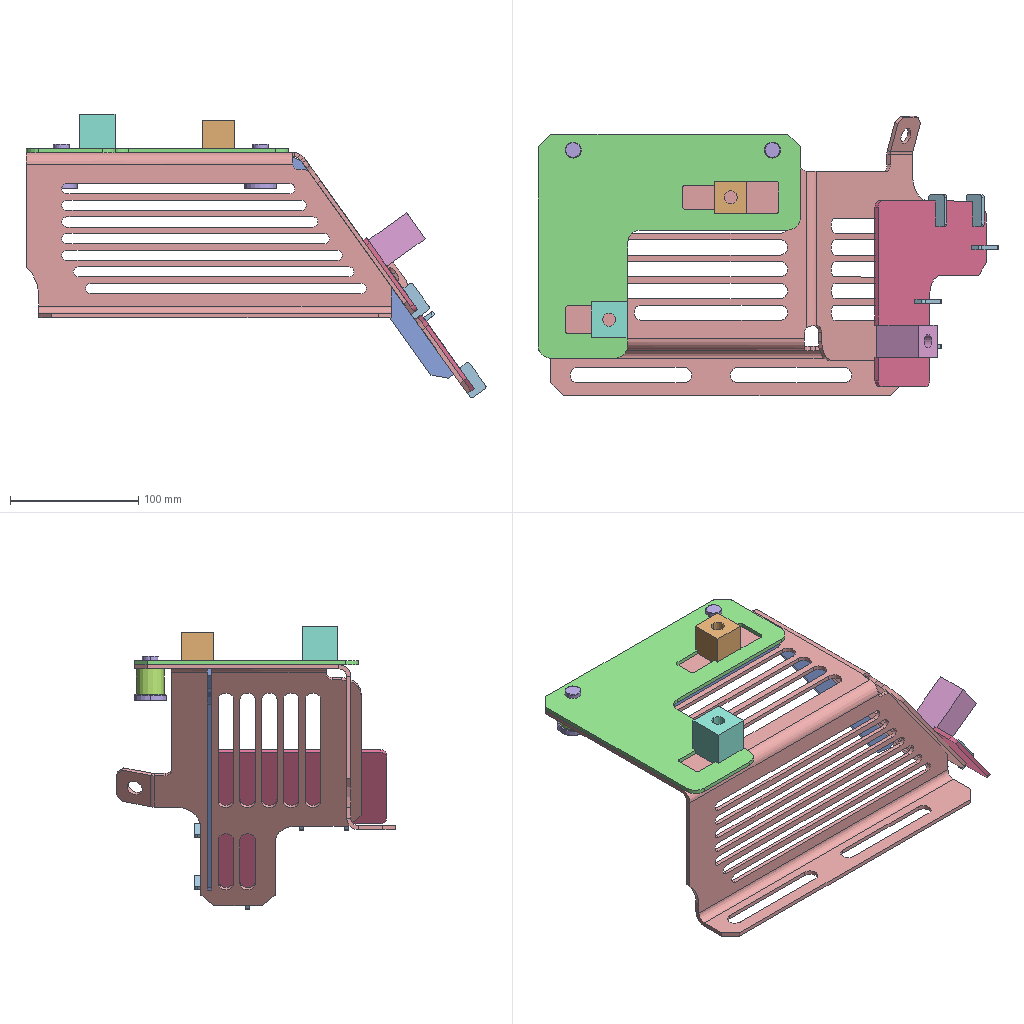Assembly | SolidWorks | 10 different items | 16 placed | box 359 x 218 x 221 mm
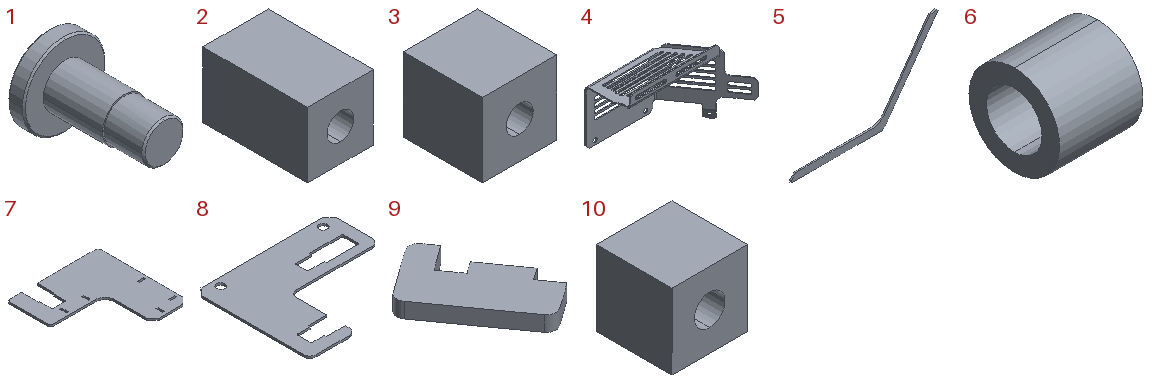Parts list (item | quantity | size | volume | features):
1 | x2 | 25 x 35 x 25 mm | 6404 mm3 | features Chamfer 1, Revolution 1
2 | x1 | 25 x 40 x 25 mm | 21731 mm3 | features FlatPattern 1, HoleWzd 1, SMBaseFlange 1, SheetMetal 1
3 | x1 | 28 x 30 x 28 mm | 21069 mm3 | features Extrusion 1, HoleWzd 1
4 | x1 | 347.398 x 187.972 x 217.987 mm | 228899 mm3 | features SM3dBend 4, FlatPattern 1, SMBaseFlange 1, SheetMetal 1
5 | x1 | 326.5 x 3.2 x 172.806 mm | 19256 mm3 | features FlatPattern 1, SMBaseFlange 1, SheetMetal 1
6 | x2 | 20 x 21.7 x 21.7 mm | 4618 mm3 | features Extrusion 1
7 | x1 | 145 x 145 x 3.2 mm | 41790 mm3 | features FlatPattern 1, SMBaseFlange 1, SheetMetal 1
8 | x1 | 205 x 175 x 3.2 mm | 60892 mm3 | features FlatPattern 1, SMBaseFlange 1, SheetMetal 1
9 | x5 | 20.748 x 27.48 x 3.2 mm | 878.159 mm3 | features FlatPattern 1, SMBaseFlange 1, SheetMetal 1
10 | x1 | 25 x 25 x 25 mm | 13582 mm3 | features Extrusion 1, HoleWzd 1
Mates (type | each side: item.copy, entity, surface, feature):
Coincident | 4.1 face plane Base-Flange1 | 5.1 face plane Base-Flange1 | 2 times
DistanceDim | 4.1 face plane Base-Flange1 | 5.1 face plane Base-Flange1
Coincident | 4.1 face plane Base-Flange1 | 6.1 face plane Boss-Extrude1
Concentric | 4.1 face cylinder Base-Flange1 | 6.1 face cylinder Boss-Extrude1
Coincident | 4.1 face plane Base-Flange1 | 6.2 face plane Boss-Extrude1
Concentric | 4.1 face cylinder Base-Flange1 | 6.2 face cylinder Boss-Extrude1
Coincident | 4.1 face plane Base-Flange1 | 2.1 face plane Base-Flange1
DistanceDim | 2.1 face plane Base-Flange1 | 4.1 face plane Base-Flange1
DistanceDim | 4.1 face plane Base-Flange1 | 2.1 face plane Base-Flange1
Coincident | 4.1 face plane Base-Flange1 | 3.1 face plane Boss-Extrude1
DistanceDim | 4.1 face plane Base-Flange1 | 3.1 face plane Boss-Extrude1
DistanceDim | 3.1 face plane Boss-Extrude1 | 4.1 face plane Base-Flange1
InPlace | 1.1 plane | assembly plane
InPlace | 4.1 face plane Base-Flange1 | 8.1 plane
InPlace | 4.1 face plane Base-Flange1 | 7.1 plane
InPlace | 9.1 plane | assembly plane
Coincident | 7.1 face plane Base-Flange1 | 9.2 face plane Base-Flange1 | 2 times
DistanceDim | 9.2 face plane Base-Flange1 | 7.1 face plane Base-Flange1
Coincident | 7.1 face plane Base-Flange1 | 9.3 face plane Base-Flange1 | 2 times
DistanceDim | 9.3 face plane Base-Flange1 | 7.1 face plane Base-Flange1
Coincident | 4.1 face plane Base-Flange1 | 10.1 face plane Boss-Extrude1
Parallel | 4.1 face plane Base-Flange1 | 10.1 face plane Boss-Extrude1
DistanceDim | 10.1 face cylinder M12 Tapped Hole1 | 4.1 face plane Base-Flange1 | 2 times